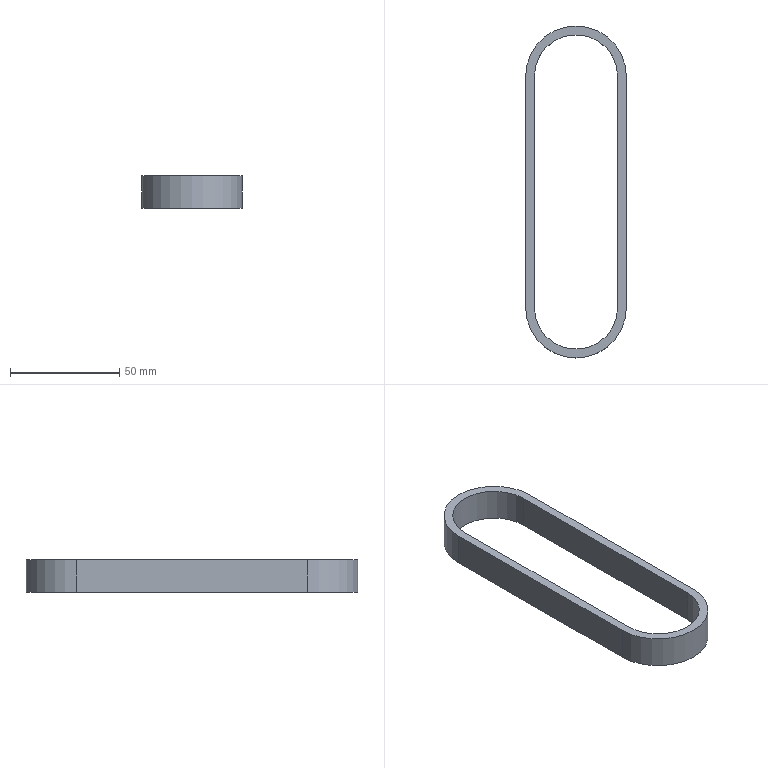Part | SolidWorks | features BeltProfileFeature 1, ExtruThin 1 | 1 solid | 10 faces | box 46.2 x 152.2 x 15 mm | volume 20675 mm3 | plane 6 | cylinder 4 | commonest cylinder face diameters 38.2 x2 46.2 x2
STEP:
#1=CARTESIAN_POINT('',(-23.1,0.,7.5));
#2=VERTEX_POINT('',#1);
#3=CARTESIAN_POINT('',(23.1,0.,7.5));
#4=VERTEX_POINT('',#3);
#5=CARTESIAN_POINT('',(0.,0.,7.5));
#6=DIRECTION('',(0.,0.,1.));
#7=DIRECTION('',(-1.,0.,0.));
#8=AXIS2_PLACEMENT_3D('',#5,#6,#7);
#9=CIRCLE('',#8,23.1);
#10=EDGE_CURVE('',#2,#4,#9,.T.);
#11=ORIENTED_EDGE('',*,*,#10,.T.);
#12=CARTESIAN_POINT('',(23.1,106.,7.5));
#13=VERTEX_POINT('',#12);
#14=CARTESIAN_POINT('',(23.1,0.,7.5));
#15=DIRECTION('',(0.,1.,0.));
#16=VECTOR('',#15,1000.);
#17=LINE('',#14,#16);
#18=EDGE_CURVE('',#4,#13,#17,.T.);
#19=ORIENTED_EDGE('',*,*,#18,.T.);
#20=CARTESIAN_POINT('',(-23.1,106.,7.5));
#21=VERTEX_POINT('',#20);
#22=CARTESIAN_POINT('',(0.,106.,7.5));
#23=DIRECTION('',(0.,0.,1.));
#24=DIRECTION('',(-1.,0.,0.));
#25=AXIS2_PLACEMENT_3D('',#22,#23,#24);
#26=CIRCLE('',#25,23.1);
#27=EDGE_CURVE('',#13,#21,#26,.T.);
#28=ORIENTED_EDGE('',*,*,#27,.T.);
#29=CARTESIAN_POINT('',(-23.1,0.,7.5));
#30=DIRECTION('',(0.,-1.,0.));
#31=VECTOR('',#30,1000.);
#32=LINE('',#29,#31);
#33=EDGE_CURVE('',#21,#2,#32,.T.);
#34=ORIENTED_EDGE('',*,*,#33,.T.);
#35=EDGE_LOOP('',(#11,#19,#28,#34));
#36=FACE_OUTER_BOUND('',#35,.T.);
#37=CARTESIAN_POINT('',(-19.1,0.,7.5));
#38=VERTEX_POINT('',#37);
#39=CARTESIAN_POINT('',(19.1,0.,7.5));
#40=VERTEX_POINT('',#39);
#41=CARTESIAN_POINT('',(0.,0.,7.5));
#42=DIRECTION('',(0.,0.,1.));
#43=DIRECTION('',(-1.,0.,0.));
#44=AXIS2_PLACEMENT_3D('',#41,#42,#43);
#45=CIRCLE('',#44,19.1);
#46=EDGE_CURVE('',#38,#40,#45,.T.);
#47=ORIENTED_EDGE('',*,*,#46,.F.);
#48=CARTESIAN_POINT('',(-19.1,106.,7.5));
#49=VERTEX_POINT('',#48);
#50=CARTESIAN_POINT('',(-19.1,0.,7.5));
#51=DIRECTION('',(0.,-1.,0.));
#52=VECTOR('',#51,1000.);
#53=LINE('',#50,#52);
#54=EDGE_CURVE('',#49,#38,#53,.T.);
#55=ORIENTED_EDGE('',*,*,#54,.F.);
#56=CARTESIAN_POINT('',(19.1,106.,7.5));
#57=VERTEX_POINT('',#56);
#58=CARTESIAN_POINT('',(0.,106.,7.5));
#59=DIRECTION('',(0.,0.,1.));
#60=DIRECTION('',(-1.,0.,0.));
#61=AXIS2_PLACEMENT_3D('',#58,#59,#60);
#62=CIRCLE('',#61,19.1);
#63=EDGE_CURVE('',#57,#49,#62,.T.);
#64=ORIENTED_EDGE('',*,*,#63,.F.);
#65=CARTESIAN_POINT('',(19.1,0.,7.5));
#66=DIRECTION('',(0.,1.,0.));
#67=VECTOR('',#66,1000.);
#68=LINE('',#65,#67);
#69=EDGE_CURVE('',#40,#57,#68,.T.);
#70=ORIENTED_EDGE('',*,*,#69,.F.);
#71=EDGE_LOOP('',(#47,#55,#64,#70));
#72=FACE_BOUND('',#71,.T.);
#73=CARTESIAN_POINT('',(0.,0.,7.5));
#74=DIRECTION('',(0.,0.,-1.));
#75=DIRECTION('',(-1.,0.,0.));
#76=AXIS2_PLACEMENT_3D('',#73,#74,#75);
#77=PLANE('',#76);
#78=ADVANCED_FACE('',(#36,#72),#77,.F.);
#79=CARTESIAN_POINT('',(-23.1,0.,-7.5));
#80=VERTEX_POINT('',#79);
#81=CARTESIAN_POINT('',(23.1,0.,-7.5));
#82=VERTEX_POINT('',#81);
#83=CARTESIAN_POINT('',(0.,0.,-7.5));
#84=DIRECTION('',(0.,0.,1.));
#85=DIRECTION('',(-1.,0.,0.));
#86=AXIS2_PLACEMENT_3D('',#83,#84,#85);
#87=CIRCLE('',#86,23.1);
#88=EDGE_CURVE('',#80,#82,#87,.T.);
#89=ORIENTED_EDGE('',*,*,#88,.F.);
#90=CARTESIAN_POINT('',(-23.1,106.,-7.5));
#91=VERTEX_POINT('',#90);
#92=CARTESIAN_POINT('',(-23.1,0.,-7.5));
#93=DIRECTION('',(0.,-1.,0.));
#94=VECTOR('',#93,1000.);
#95=LINE('',#92,#94);
#96=EDGE_CURVE('',#91,#80,#95,.T.);
#97=ORIENTED_EDGE('',*,*,#96,.F.);
#98=CARTESIAN_POINT('',(23.1,106.,-7.5));
#99=VERTEX_POINT('',#98);
#100=CARTESIAN_POINT('',(0.,106.,-7.5));
#101=DIRECTION('',(0.,0.,1.));
#102=DIRECTION('',(-1.,0.,0.));
#103=AXIS2_PLACEMENT_3D('',#100,#101,#102);
#104=CIRCLE('',#103,23.1);
#105=EDGE_CURVE('',#99,#91,#104,.T.);
#106=ORIENTED_EDGE('',*,*,#105,.F.);
#107=CARTESIAN_POINT('',(23.1,0.,-7.5));
#108=DIRECTION('',(0.,1.,0.));
#109=VECTOR('',#108,1000.);
#110=LINE('',#107,#109);
#111=EDGE_CURVE('',#82,#99,#110,.T.);
#112=ORIENTED_EDGE('',*,*,#111,.F.);
#113=EDGE_LOOP('',(#89,#97,#106,#112));
#114=FACE_OUTER_BOUND('',#113,.T.);
#115=CARTESIAN_POINT('',(-19.1,106.,-7.5));
#116=VERTEX_POINT('',#115);
#117=CARTESIAN_POINT('',(-19.1,0.,-7.5));
#118=VERTEX_POINT('',#117);
#119=CARTESIAN_POINT('',(-19.1,0.,-7.5));
#120=DIRECTION('',(0.,-1.,0.));
#121=VECTOR('',#120,1000.);
#122=LINE('',#119,#121);
#123=EDGE_CURVE('',#116,#118,#122,.T.);
#124=ORIENTED_EDGE('',*,*,#123,.T.);
#125=CARTESIAN_POINT('',(19.1,0.,-7.5));
#126=VERTEX_POINT('',#125);
#127=CARTESIAN_POINT('',(0.,0.,-7.5));
#128=DIRECTION('',(0.,0.,1.));
#129=DIRECTION('',(-1.,0.,0.));
#130=AXIS2_PLACEMENT_3D('',#127,#128,#129);
#131=CIRCLE('',#130,19.1);
#132=EDGE_CURVE('',#118,#126,#131,.T.);
#133=ORIENTED_EDGE('',*,*,#132,.T.);
#134=CARTESIAN_POINT('',(19.1,106.,-7.5));
#135=VERTEX_POINT('',#134);
#136=CARTESIAN_POINT('',(19.1,0.,-7.5));
#137=DIRECTION('',(0.,1.,0.));
#138=VECTOR('',#137,1000.);
#139=LINE('',#136,#138);
#140=EDGE_CURVE('',#126,#135,#139,.T.);
#141=ORIENTED_EDGE('',*,*,#140,.T.);
#142=CARTESIAN_POINT('',(0.,106.,-7.5));
#143=DIRECTION('',(0.,0.,1.));
#144=DIRECTION('',(-1.,0.,0.));
#145=AXIS2_PLACEMENT_3D('',#142,#143,#144);
#146=CIRCLE('',#145,19.1);
#147=EDGE_CURVE('',#135,#116,#146,.T.);
#148=ORIENTED_EDGE('',*,*,#147,.T.);
#149=EDGE_LOOP('',(#124,#133,#141,#148));
#150=FACE_BOUND('',#149,.T.);
#151=CARTESIAN_POINT('',(0.,0.,-7.5));
#152=DIRECTION('',(0.,0.,-1.));
#153=DIRECTION('',(-1.,0.,0.));
#154=AXIS2_PLACEMENT_3D('',#151,#152,#153);
#155=PLANE('',#154);
#156=ADVANCED_FACE('',(#114,#150),#155,.T.);
#157=ORIENTED_EDGE('',*,*,#88,.T.);
#158=CARTESIAN_POINT('',(23.1,0.,7.5));
#159=DIRECTION('',(0.,0.,-1.));
#160=VECTOR('',#159,1000.);
#161=LINE('',#158,#160);
#162=EDGE_CURVE('',#4,#82,#161,.T.);
#163=ORIENTED_EDGE('',*,*,#162,.F.);
#164=ORIENTED_EDGE('',*,*,#10,.F.);
#165=CARTESIAN_POINT('',(-23.1,0.,7.5));
#166=DIRECTION('',(0.,0.,-1.));
#167=VECTOR('',#166,1000.);
#168=LINE('',#165,#167);
#169=EDGE_CURVE('',#2,#80,#168,.T.);
#170=ORIENTED_EDGE('',*,*,#169,.T.);
#171=EDGE_LOOP('',(#157,#163,#164,#170));
#172=FACE_OUTER_BOUND('',#171,.T.);
#173=CARTESIAN_POINT('',(0.,0.,7.5));
#174=DIRECTION('',(0.,0.,-1.));
#175=DIRECTION('',(-1.,0.,0.));
#176=AXIS2_PLACEMENT_3D('',#173,#174,#175);
#177=CYLINDRICAL_SURFACE('',#176,23.1);
#178=ADVANCED_FACE('',(#172),#177,.T.);
#179=ORIENTED_EDGE('',*,*,#111,.T.);
#180=CARTESIAN_POINT('',(23.1,106.,7.5));
#181=DIRECTION('',(0.,0.,-1.));
#182=VECTOR('',#181,1000.);
#183=LINE('',#180,#182);
#184=EDGE_CURVE('',#13,#99,#183,.T.);
#185=ORIENTED_EDGE('',*,*,#184,.F.);
#186=ORIENTED_EDGE('',*,*,#18,.F.);
#187=ORIENTED_EDGE('',*,*,#162,.T.);
#188=EDGE_LOOP('',(#179,#185,#186,#187));
#189=FACE_OUTER_BOUND('',#188,.T.);
#190=CARTESIAN_POINT('',(23.1,0.,7.5));
#191=DIRECTION('',(-1.,0.,0.));
#192=DIRECTION('',(0.,-1.,0.));
#193=AXIS2_PLACEMENT_3D('',#190,#191,#192);
#194=PLANE('',#193);
#195=ADVANCED_FACE('',(#189),#194,.F.);
#196=ORIENTED_EDGE('',*,*,#105,.T.);
#197=CARTESIAN_POINT('',(-23.1,106.,7.5));
#198=DIRECTION('',(0.,0.,-1.));
#199=VECTOR('',#198,1000.);
#200=LINE('',#197,#199);
#201=EDGE_CURVE('',#21,#91,#200,.T.);
#202=ORIENTED_EDGE('',*,*,#201,.F.);
#203=ORIENTED_EDGE('',*,*,#27,.F.);
#204=ORIENTED_EDGE('',*,*,#184,.T.);
#205=EDGE_LOOP('',(#196,#202,#203,#204));
#206=FACE_OUTER_BOUND('',#205,.T.);
#207=CARTESIAN_POINT('',(0.,106.,7.5));
#208=DIRECTION('',(0.,0.,-1.));
#209=DIRECTION('',(-1.,0.,0.));
#210=AXIS2_PLACEMENT_3D('',#207,#208,#209);
#211=CYLINDRICAL_SURFACE('',#210,23.1);
#212=ADVANCED_FACE('',(#206),#211,.T.);
#213=ORIENTED_EDGE('',*,*,#96,.T.);
#214=ORIENTED_EDGE('',*,*,#169,.F.);
#215=ORIENTED_EDGE('',*,*,#33,.F.);
#216=ORIENTED_EDGE('',*,*,#201,.T.);
#217=EDGE_LOOP('',(#213,#214,#215,#216));
#218=FACE_OUTER_BOUND('',#217,.T.);
#219=CARTESIAN_POINT('',(-23.1,0.,7.5));
#220=DIRECTION('',(1.,0.,0.));
#221=DIRECTION('',(0.,1.,0.));
#222=AXIS2_PLACEMENT_3D('',#219,#220,#221);
#223=PLANE('',#222);
#224=ADVANCED_FACE('',(#218),#223,.F.);
#225=ORIENTED_EDGE('',*,*,#132,.F.);
#226=CARTESIAN_POINT('',(-19.1,0.,7.5));
#227=DIRECTION('',(0.,0.,-1.));
#228=VECTOR('',#227,1000.);
#229=LINE('',#226,#228);
#230=EDGE_CURVE('',#38,#118,#229,.T.);
#231=ORIENTED_EDGE('',*,*,#230,.F.);
#232=ORIENTED_EDGE('',*,*,#46,.T.);
#233=CARTESIAN_POINT('',(19.1,0.,7.5));
#234=DIRECTION('',(0.,0.,-1.));
#235=VECTOR('',#234,1000.);
#236=LINE('',#233,#235);
#237=EDGE_CURVE('',#40,#126,#236,.T.);
#238=ORIENTED_EDGE('',*,*,#237,.T.);
#239=EDGE_LOOP('',(#225,#231,#232,#238));
#240=FACE_OUTER_BOUND('',#239,.T.);
#241=CARTESIAN_POINT('',(0.,0.,7.5));
#242=DIRECTION('',(0.,0.,-1.));
#243=DIRECTION('',(-1.,0.,0.));
#244=AXIS2_PLACEMENT_3D('',#241,#242,#243);
#245=CYLINDRICAL_SURFACE('',#244,19.1);
#246=ADVANCED_FACE('',(#240),#245,.F.);
#247=ORIENTED_EDGE('',*,*,#140,.F.);
#248=ORIENTED_EDGE('',*,*,#237,.F.);
#249=ORIENTED_EDGE('',*,*,#69,.T.);
#250=CARTESIAN_POINT('',(19.1,106.,7.5));
#251=DIRECTION('',(0.,0.,-1.));
#252=VECTOR('',#251,1000.);
#253=LINE('',#250,#252);
#254=EDGE_CURVE('',#57,#135,#253,.T.);
#255=ORIENTED_EDGE('',*,*,#254,.T.);
#256=EDGE_LOOP('',(#247,#248,#249,#255));
#257=FACE_OUTER_BOUND('',#256,.T.);
#258=CARTESIAN_POINT('',(19.1,0.,7.5));
#259=DIRECTION('',(-1.,0.,0.));
#260=DIRECTION('',(0.,-1.,0.));
#261=AXIS2_PLACEMENT_3D('',#258,#259,#260);
#262=PLANE('',#261);
#263=ADVANCED_FACE('',(#257),#262,.T.);
#264=ORIENTED_EDGE('',*,*,#147,.F.);
#265=ORIENTED_EDGE('',*,*,#254,.F.);
#266=ORIENTED_EDGE('',*,*,#63,.T.);
#267=CARTESIAN_POINT('',(-19.1,106.,7.5));
#268=DIRECTION('',(0.,0.,-1.));
#269=VECTOR('',#268,1000.);
#270=LINE('',#267,#269);
#271=EDGE_CURVE('',#49,#116,#270,.T.);
#272=ORIENTED_EDGE('',*,*,#271,.T.);
#273=EDGE_LOOP('',(#264,#265,#266,#272));
#274=FACE_OUTER_BOUND('',#273,.T.);
#275=CARTESIAN_POINT('',(0.,106.,7.5));
#276=DIRECTION('',(0.,0.,-1.));
#277=DIRECTION('',(-1.,0.,0.));
#278=AXIS2_PLACEMENT_3D('',#275,#276,#277);
#279=CYLINDRICAL_SURFACE('',#278,19.1);
#280=ADVANCED_FACE('',(#274),#279,.F.);
#281=ORIENTED_EDGE('',*,*,#123,.F.);
#282=ORIENTED_EDGE('',*,*,#271,.F.);
#283=ORIENTED_EDGE('',*,*,#54,.T.);
#284=ORIENTED_EDGE('',*,*,#230,.T.);
#285=EDGE_LOOP('',(#281,#282,#283,#284));
#286=FACE_OUTER_BOUND('',#285,.T.);
#287=CARTESIAN_POINT('',(-19.1,0.,7.5));
#288=DIRECTION('',(1.,0.,0.));
#289=DIRECTION('',(0.,1.,0.));
#290=AXIS2_PLACEMENT_3D('',#287,#288,#289);
#291=PLANE('',#290);
#292=ADVANCED_FACE('',(#286),#291,.T.);
#293=CLOSED_SHELL('',(#78,#156,#178,#195,#212,#224,#246,#263,#280,#292));
#294=MANIFOLD_SOLID_BREP('',#293);
#295=CARTESIAN_POINT('',(0.,0.,0.));
#296=DIRECTION('',(0.,0.,1.));
#297=DIRECTION('',(1.,0.,0.));
#298=AXIS2_PLACEMENT_3D('',#295,#296,#297);
#299=(LENGTH_UNIT()NAMED_UNIT(*)SI_UNIT(.MILLI.,.METRE.));
#300=UNCERTAINTY_MEASURE_WITH_UNIT(LENGTH_MEASURE(0.00001),#299,'','');
#301=(NAMED_UNIT(*)PLANE_ANGLE_UNIT()SI_UNIT($,.RADIAN.));
#302=(NAMED_UNIT(*)SI_UNIT($,.STERADIAN.)SOLID_ANGLE_UNIT());
#303=(GEOMETRIC_REPRESENTATION_CONTEXT(3)GLOBAL_UNCERTAINTY_ASSIGNED_CONTEXT((#300))GLOBAL_UNIT_ASSIGNED_CONTEXT((#299,#301,#302))REPRESENTATION_CONTEXT('',''));
#304=ADVANCED_BREP_SHAPE_REPRESENTATION('',(#294,#298),#303);